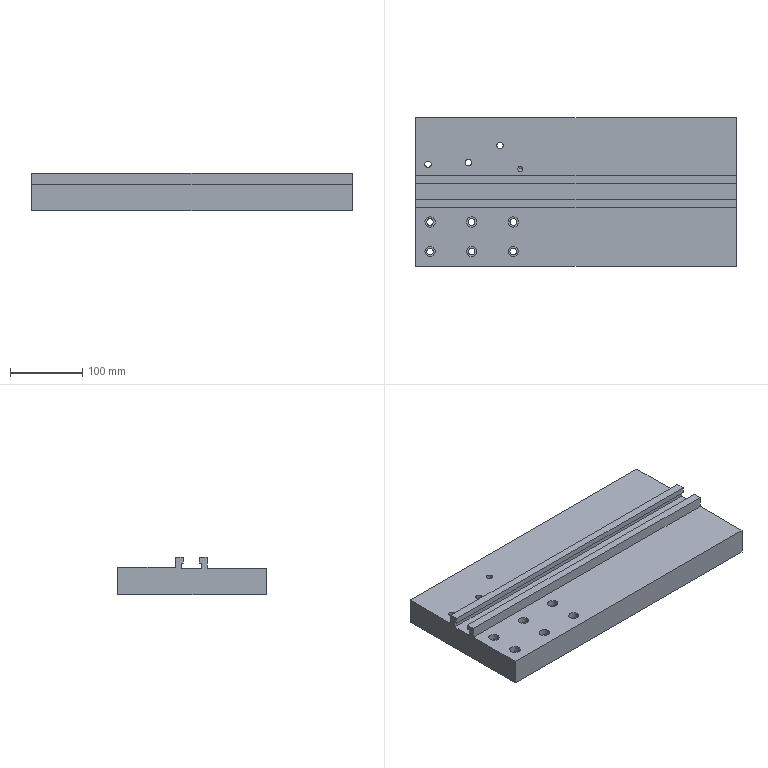Part | Creo | 1 solid | 74 faces | box 444 x 206.013 x 51.606 mm | volume 3465438 mm3 | cylinder 38 | plane 28 | cone 8 | commonest cylinder face diameters 9 x18 14.25 x12 8.782 x6 6.985 x2